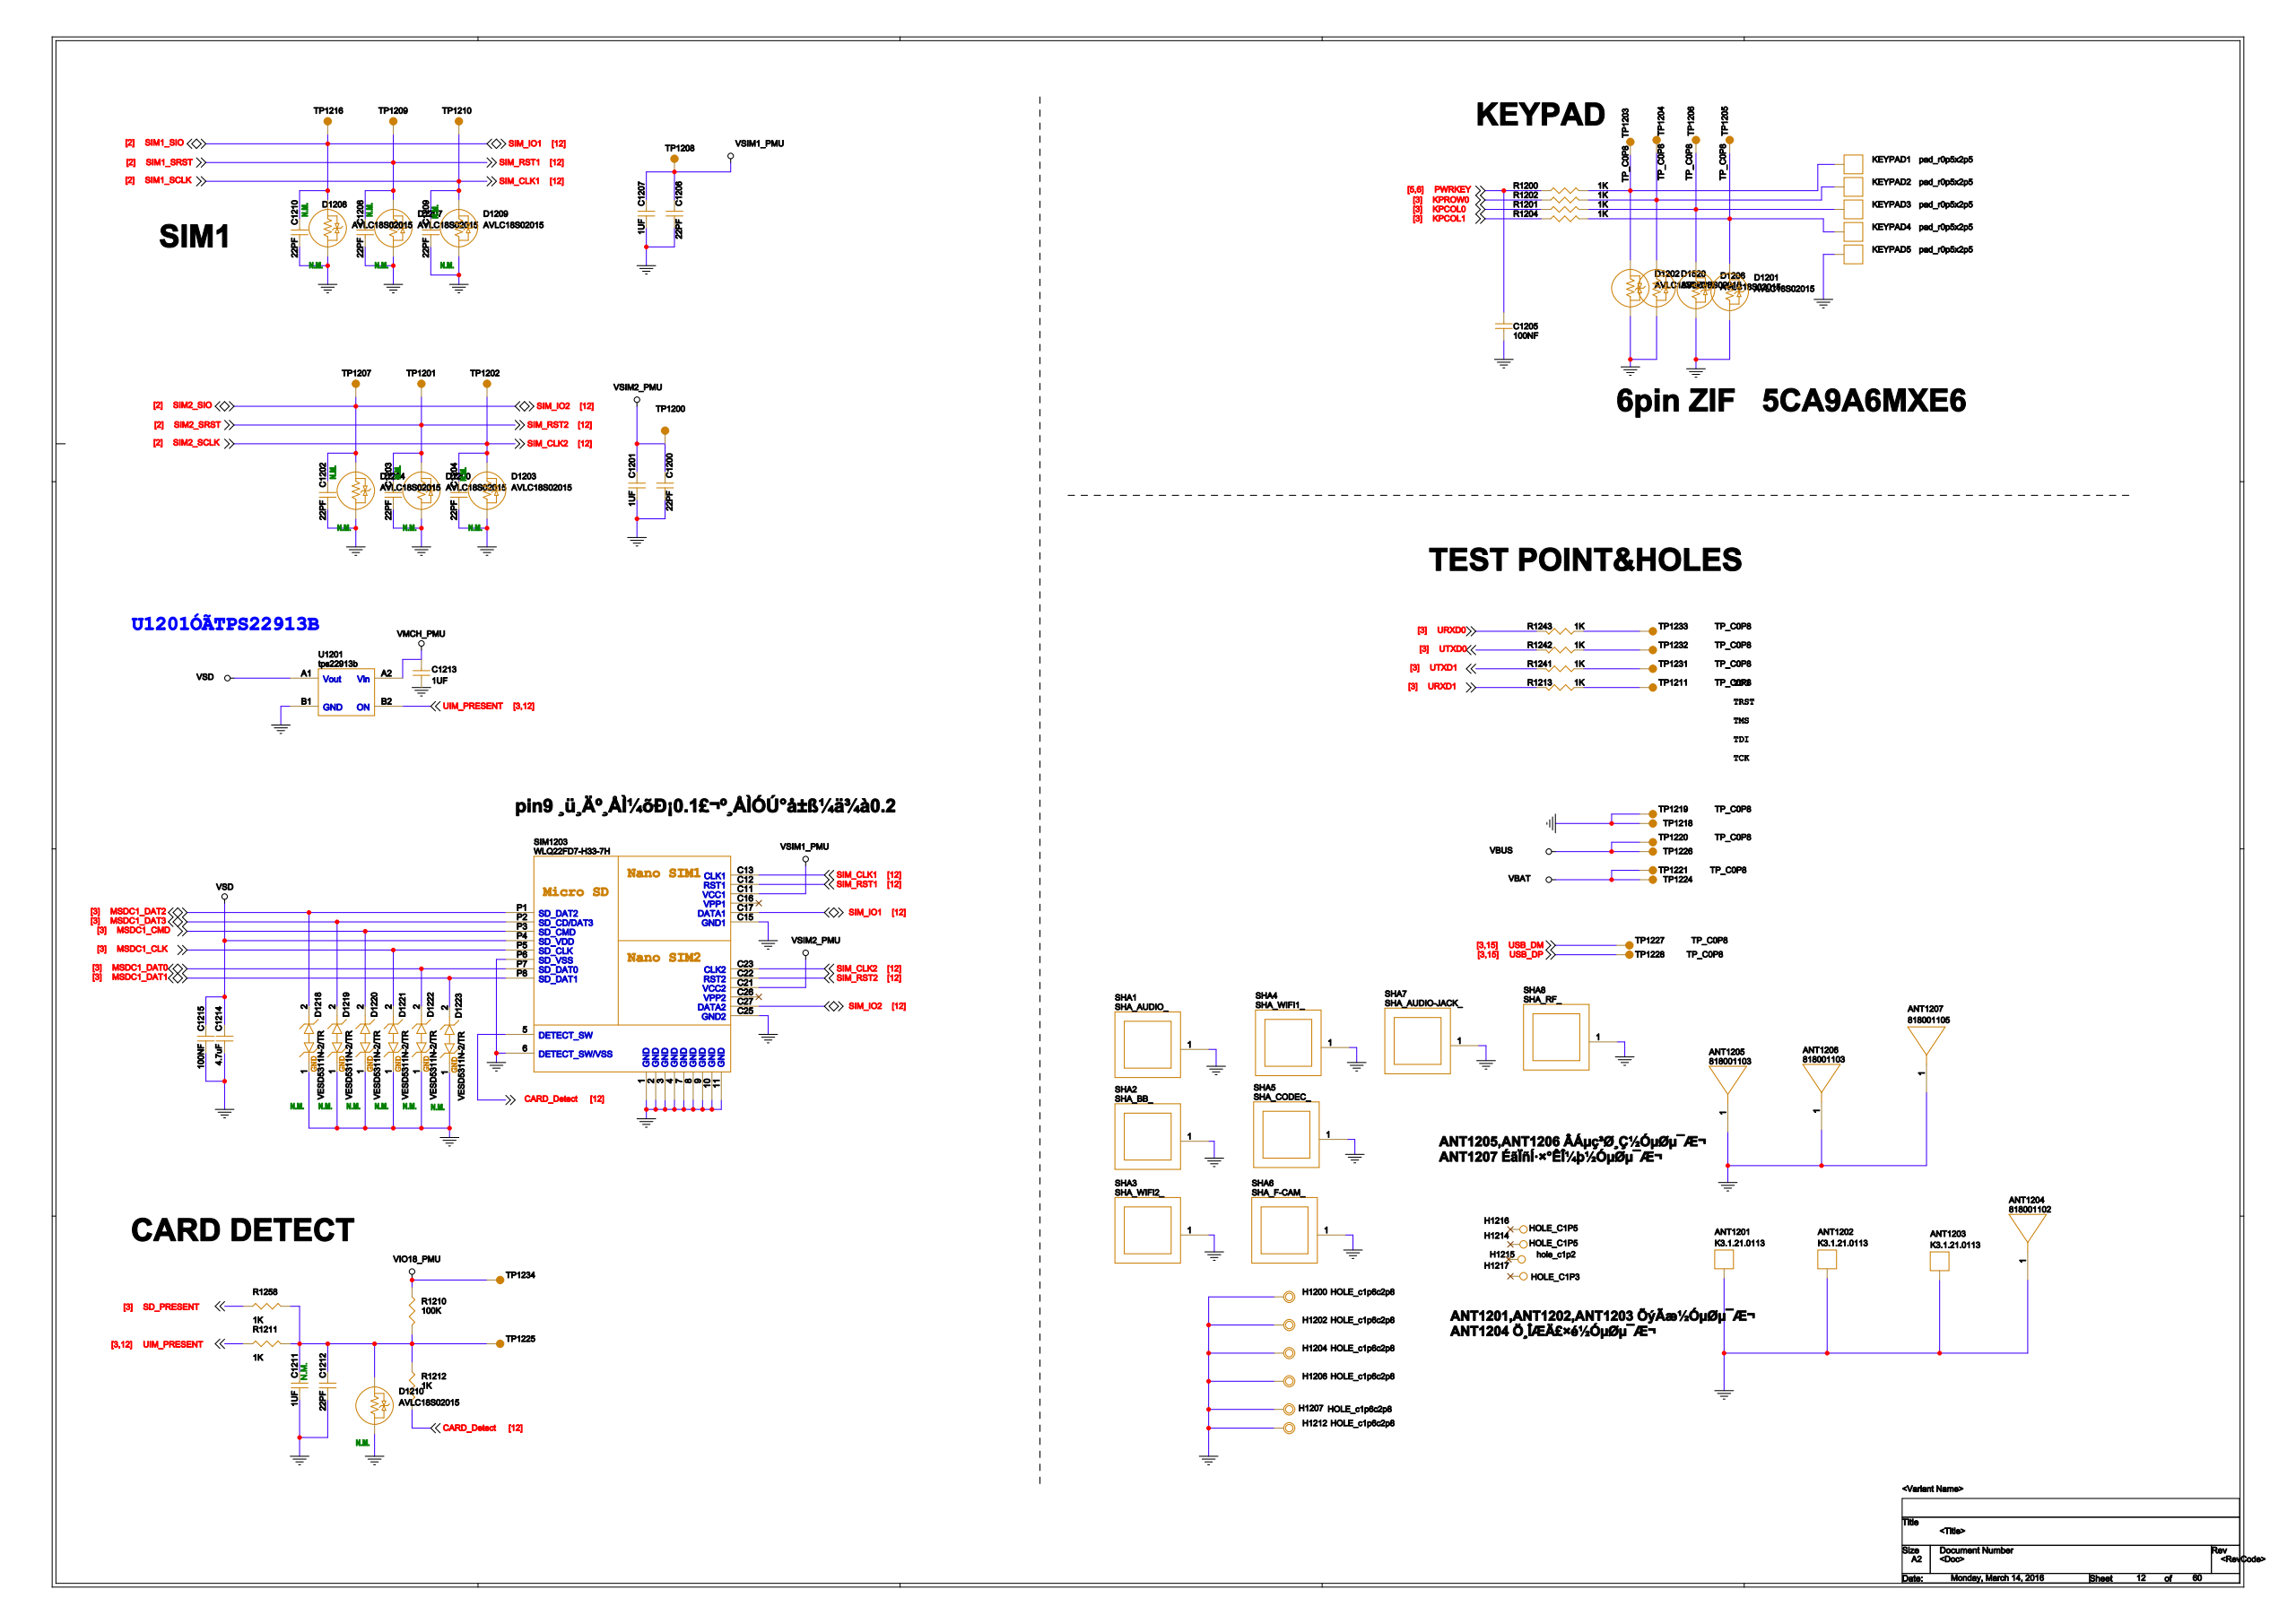Circuit board | Cadence Allegro | 1088 parts | 793 nets | one sheet of the schematic
Parts on this sheet (reference | value | footprint):
ANT1201 | K3.1.21.0113 | PIN_ANT_K3_1_21_0113
ANT1202 | K3.1.21.0113 | PIN_ANT_K3_1_21_0113
ANT1203 | K3.1.21.0113 | PIN_ANT_K3_1_21_0113
ANT1204 | 818001102 | PIN_ANT_818001102
ANT1205 | 818001103 | PIN_ANT_818001103
ANT1206 | 818001103 | PIN_ANT_818001103
ANT1207 | 818001105 | PIN_ANT_818001105
C1200 | 22PF | C0201
C1201 | 1UF | C0201
C1202
C1203
C1204
C1205 | 100NF | C0201
C1206 | 22PF | C0201
C1207 | 1UF | C0201
C1208
C1209
C1210
C1211
C1212 | 22PF | C0201
C1213 | 1UF | C0201
C1214 | 4.7uF | 0402-BIG
C1215 | 100NF | C0201
D1200
D1201 | AVLC18S02015 | R0402_H0P7
D1202 | AVLC18S02015 | R0402_H0P7
D1203
D1204
D1206 | AVLC18S02015 | R0402_H0P7
D1207
D1208
D1209
D1210
D1218
D1219
D1220
D1221
D1222
D1223
D1520 | AVLC18S02015 | R0402_H0P7
H1200 | HOLE_c1p6c2p8 | HOLE_C1P6C2P8
H1202 | HOLE_c1p6c2p8 | HOLE_C1P6C2P8
H1204 | HOLE_c1p6c2p8 | HOLE_C1P6C2P8
H1206 | HOLE_c1p6c2p8 | HOLE_C1P6C2P8
H1207 | HOLE_c1p6c2p8 | HOLE_C1P6C2P8
H1212 | HOLE_c1p6c2p8 | HOLE_C1P6C2P8
KEYPAD1 | pad_r0p5x2p5 | PAD_R0P5X2P5
KEYPAD2 | pad_r0p5x2p5 | PAD_R0P5X2P5
KEYPAD3 | pad_r0p5x2p5 | PAD_R0P5X2P5
KEYPAD4 | pad_r0p5x2p5 | PAD_R0P5X2P5
KEYPAD5 | pad_r0p5x2p5 | PAD_R0P5X2P5
R1200 | 1K | R0201
R1201 | 1K | R0201
R1202 | 1K | R0201
R1204 | 1K | R0201
R1210 | 100K | R0201
R1211 | 1K | R0201
R1212 | 1K | R0201
R1213 | 1K | R0201
R1241 | 1K | R0201
R1242 | 1K | R0201
R1243 | 1K | R0201
R1258 | 1K | R0201
SHA1 | SHA_AUDIO_xxx | SHA_AUDIO_xxx
SHA2 | SHA_BB_xxx | SHA_BB_xxx
SHA3 | SHA_WIFI2_xxx | SHA_WIFI2_xxx
SHA4 | SHA_WIFI1_xxx | SHA_WIFI1_xxx
SHA5 | SHA_CODEC_xxx | SHA_CODEC_xxx
SHA6 | SHA_F-CAM_xxx | SHA_F-CAM_xxx
SHA7 | SHA_AUDIO-JACK_xxx | SHA_AUDIO-JACK_xxx
SHA8 | SHA_RF_xxx | SHA_RF_xxx
SIM1203 | WLQ22FD7-H33-7H | SIM_WLQ22FD7-H33-7H
TP1200 | TP_C0P8 | TP_C0P8
TP1201 | TP_C0P8 | TP_C0P8
TP1202 | TP_C0P8 | TP_C0P8
TP1203 | TP_C0P8 | TP_C0P8
TP1204 | TP_C0P8 | TP_C0P8
TP1205 | TP_C0P8 | TP_C0P8
TP1206 | TP_C0P8 | TP_C0P8
TP1207 | TP_C0P8 | TP_C0P8
TP1208 | TP_C0P8 | TP_C0P8
TP1209 | TP_C0P8 | TP_C0P8
TP1210 | TP_C0P8 | TP_C0P8
TP1211 | TP_C0P8 | TP_C0P8
TP1216 | TP_C0P8 | TP_C0P8
TP1218 | TP_C0P8 | TP_C0P8
TP1219 | TP_C0P8 | TP_C0P8
TP1220 | TP_C0P8 | TP_C0P8
TP1221 | TP_C0P8 | TP_C0P8
TP1224 | TP_C0P8 | TP_C0P8
TP1225 | TP_C0P8 | TP_C0P8
TP1226 | TP_C0P8 | TP_C0P8
TP1227 | TP_C0P8 | TP_C0P8
TP1228 | TP_C0P8 | TP_C0P8
TP1231 | TP_C0P8 | TP_C0P8
TP1232 | TP_C0P8 | TP_C0P8
TP1233 | TP_C0P8 | TP_C0P8
TP1234 | TP_C0P8 | TP_C0P8
U1201 | tps22913b | CSP4_0P888X0P888X0P6_0P5
Nets of these parts (net: part-pin ...):
GND: ANT1201-1 ANT1202-1 ANT1203-1 ANT1204-1 ANT1205-1 ANT1206-1 ANT1207-1 C1200-2 C1201-2 C1202-2 C1203-2 C1204-2 C1205-2 C1206-2 C1207-2 C1208-2 C1209-2 C1210-2 C1211-2 C1212-2 C1213-2 C1214-2 C1215-2 D1200-2 D1201-2 D1202-2 D1203-2 D1204-2 D1206-2 D1207-2 D1208-2 D1209-2 D1210-2 D1218-1 D1219-1 D1220-1 D1221-1 D1222-1 D1223-1 D1520-2 H1200-1 H1202-1 H1204-1 H1206-1 H1207-1 H1212-1 KEYPAD5-1 SHA1-1 SHA2-1 SHA3-1 SHA4-1 SHA5-1 SHA6-1 SHA7-1 SHA8-1 TP1218-1 TP1219-1 U1201-B1 SIM1203-1 SIM1203-2 SIM1203-3 SIM1203-4 SIM1203-6 SIM1203-7 SIM1203-8 SIM1203-9 SIM1203-10 SIM1203-11 SIM1203-C15 SIM1203-C25 SIM1203-P6
VBAT: TP1221-1 TP1224-1
SIM1_SCLK: C1209-1 D1209-1 TP1210-1 SIM1203-C13
SIM1_SIO: C1210-1 D1208-1 TP1216-1 SIM1203-C17
SIM1_SRST: C1208-1 D1207-1 TP1209-1 SIM1203-C12
SIM2_SCLK: C1204-1 D1203-1 TP1202-1 SIM1203-C23
SIM2_SIO: C1202-1 D1204-1 TP1207-1 SIM1203-C27
SIM2_SRST: C1203-1 D1200-1 TP1201-1 SIM1203-C22
URXD1: R1213-2
UTXD1: R1241-2
SD_PRESENT: R1258-1
UIM_PRESENT: R1211-1 U1201-B2
KPCOL0: R1201-1
KPCOL1: R1204-1
KPROW0: R1202-1
MSDC1_CMD: D1220-2 SIM1203-P3
MSDC1_DAT0: D1222-2 SIM1203-P7
MSDC1_DAT1: D1223-2 SIM1203-P8
MSDC1_DAT2: D1218-2 SIM1203-P1
MSDC1_DAT3: D1219-2 SIM1203-P2
URXD0: R1243-2
USB_DM: TP1227-1
USB_DP: TP1228-1
UTXD0: R1242-2
VIO18_PMU: R1210-1 TP1234-1
VSIM1_PMU: C1206-1 C1207-1 TP1208-1 SIM1203-C11
VSIM2_PMU: C1200-1 C1201-1 TP1200-1 SIM1203-C21
N33359700: D1201-1 KEYPAD4-1 R1204-2 TP1205-1
N18533203: D1202-1 KEYPAD1-1 R1200-2 TP1203-1
N33359693: D1206-1 KEYPAD3-1 R1201-2 TP1206-1
N34189732: C1211-1 C1212-1 D1210-1 R1210-2 R1211-2 R1212-1 R1258-2 TP1225-1
N18533210: D1520-1 KEYPAD2-1 R1202-2 TP1204-1
CARD_DETECT: R1212-2 SIM1203-5
MSDC1_CLK: D1221-2 SIM1203-P5
VSD: C1214-1 C1215-1 U1201-A1 SIM1203-P4
VBUS: TP1220-1 TP1226-1
VMCH_PMU: C1213-1 U1201-A2
PWRKEY: C1205-1 R1200-1
N38678504: R1213-1 TP1211-1
N32021763: R1241-1 TP1231-1
N32021762: R1242-1 TP1232-1
N32021761: R1243-1 TP1233-1